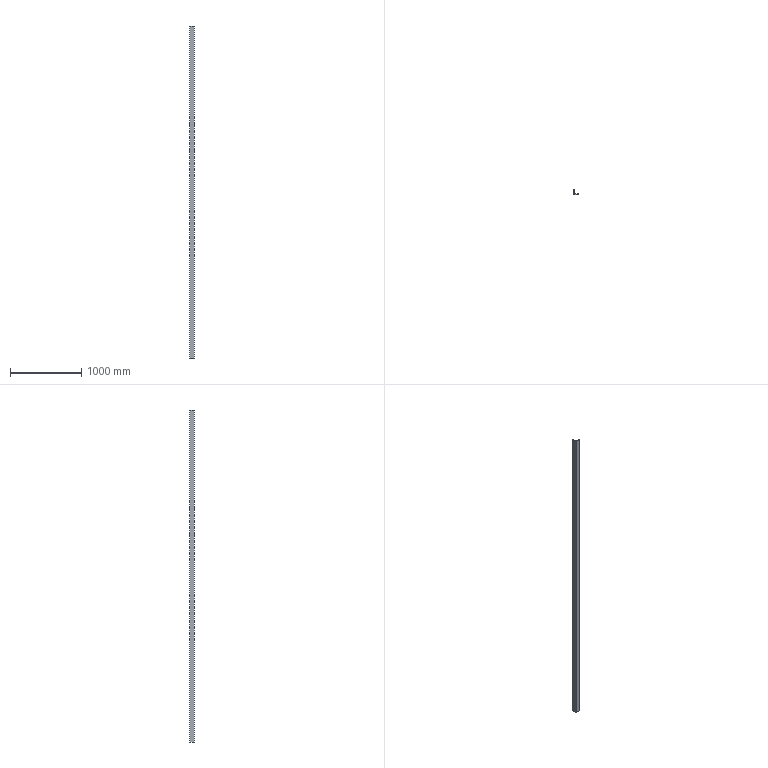Part | SolidWorks | features Extrusion 1 | 1 solid | 11 faces | box 70 x 70 x 4660 mm | volume 4966962 mm3 | plane 8 | cylinder 3 | commonest cylinder face diameters 6 x2 16 x1
STEP:
#1=CARTESIAN_POINT('',(5.,70.,0.));
#2=VERTEX_POINT('',#1);
#3=CARTESIAN_POINT('',(0.,70.,0.));
#4=VERTEX_POINT('',#3);
#5=CARTESIAN_POINT('',(5.,70.,0.));
#6=DIRECTION('',(-1.,0.,0.));
#7=VECTOR('',#6,1000.);
#8=LINE('',#5,#7);
#9=EDGE_CURVE('',#2,#4,#8,.T.);
#10=ORIENTED_EDGE('',*,*,#9,.T.);
#11=CARTESIAN_POINT('',(0.,70.,4660.));
#12=VERTEX_POINT('',#11);
#13=CARTESIAN_POINT('',(0.,70.,4660.));
#14=DIRECTION('',(0.,0.,-1.));
#15=VECTOR('',#14,1000.);
#16=LINE('',#13,#15);
#17=EDGE_CURVE('',#12,#4,#16,.T.);
#18=ORIENTED_EDGE('',*,*,#17,.F.);
#19=CARTESIAN_POINT('',(5.,70.,4660.));
#20=VERTEX_POINT('',#19);
#21=CARTESIAN_POINT('',(5.,70.,4660.));
#22=DIRECTION('',(-1.,0.,0.));
#23=VECTOR('',#22,1000.);
#24=LINE('',#21,#23);
#25=EDGE_CURVE('',#20,#12,#24,.T.);
#26=ORIENTED_EDGE('',*,*,#25,.F.);
#27=CARTESIAN_POINT('',(5.,70.,4660.));
#28=DIRECTION('',(0.,0.,-1.));
#29=VECTOR('',#28,1000.);
#30=LINE('',#27,#29);
#31=EDGE_CURVE('',#20,#2,#30,.T.);
#32=ORIENTED_EDGE('',*,*,#31,.T.);
#33=EDGE_LOOP('',(#10,#18,#26,#32));
#34=FACE_OUTER_BOUND('',#33,.T.);
#35=CARTESIAN_POINT('',(5.,70.,4660.));
#36=DIRECTION('',(0.,-1.,0.));
#37=DIRECTION('',(0.,0.,-1.));
#38=AXIS2_PLACEMENT_3D('',#35,#36,#37);
#39=PLANE('',#38);
#40=ADVANCED_FACE('',(#34),#39,.F.);
#41=CARTESIAN_POINT('',(0.,0.,0.));
#42=VERTEX_POINT('',#41);
#43=CARTESIAN_POINT('',(0.,70.,0.));
#44=DIRECTION('',(0.,-1.,0.));
#45=VECTOR('',#44,1000.);
#46=LINE('',#43,#45);
#47=EDGE_CURVE('',#4,#42,#46,.T.);
#48=ORIENTED_EDGE('',*,*,#47,.T.);
#49=CARTESIAN_POINT('',(0.,0.,4660.));
#50=VERTEX_POINT('',#49);
#51=CARTESIAN_POINT('',(0.,0.,4660.));
#52=DIRECTION('',(0.,0.,-1.));
#53=VECTOR('',#52,1000.);
#54=LINE('',#51,#53);
#55=EDGE_CURVE('',#50,#42,#54,.T.);
#56=ORIENTED_EDGE('',*,*,#55,.F.);
#57=CARTESIAN_POINT('',(0.,70.,4660.));
#58=DIRECTION('',(0.,-1.,0.));
#59=VECTOR('',#58,1000.);
#60=LINE('',#57,#59);
#61=EDGE_CURVE('',#12,#50,#60,.T.);
#62=ORIENTED_EDGE('',*,*,#61,.F.);
#63=ORIENTED_EDGE('',*,*,#17,.T.);
#64=EDGE_LOOP('',(#48,#56,#62,#63));
#65=FACE_OUTER_BOUND('',#64,.T.);
#66=CARTESIAN_POINT('',(0.,70.,4660.));
#67=DIRECTION('',(1.,0.,0.));
#68=DIRECTION('',(0.,0.,-1.));
#69=AXIS2_PLACEMENT_3D('',#66,#67,#68);
#70=PLANE('',#69);
#71=ADVANCED_FACE('',(#65),#70,.F.);
#72=CARTESIAN_POINT('',(70.,0.,0.));
#73=VERTEX_POINT('',#72);
#74=CARTESIAN_POINT('',(0.,0.,0.));
#75=DIRECTION('',(1.,0.,0.));
#76=VECTOR('',#75,1000.);
#77=LINE('',#74,#76);
#78=EDGE_CURVE('',#42,#73,#77,.T.);
#79=ORIENTED_EDGE('',*,*,#78,.T.);
#80=CARTESIAN_POINT('',(70.,0.,4660.));
#81=VERTEX_POINT('',#80);
#82=CARTESIAN_POINT('',(70.,0.,4660.));
#83=DIRECTION('',(0.,0.,-1.));
#84=VECTOR('',#83,1000.);
#85=LINE('',#82,#84);
#86=EDGE_CURVE('',#81,#73,#85,.T.);
#87=ORIENTED_EDGE('',*,*,#86,.F.);
#88=CARTESIAN_POINT('',(0.,0.,4660.));
#89=DIRECTION('',(1.,0.,0.));
#90=VECTOR('',#89,1000.);
#91=LINE('',#88,#90);
#92=EDGE_CURVE('',#50,#81,#91,.T.);
#93=ORIENTED_EDGE('',*,*,#92,.F.);
#94=ORIENTED_EDGE('',*,*,#55,.T.);
#95=EDGE_LOOP('',(#79,#87,#93,#94));
#96=FACE_OUTER_BOUND('',#95,.T.);
#97=CARTESIAN_POINT('',(0.,0.,4660.));
#98=DIRECTION('',(0.,1.,0.));
#99=DIRECTION('',(0.,0.,1.));
#100=AXIS2_PLACEMENT_3D('',#97,#98,#99);
#101=PLANE('',#100);
#102=ADVANCED_FACE('',(#96),#101,.F.);
#103=CARTESIAN_POINT('',(70.,5.,0.));
#104=VERTEX_POINT('',#103);
#105=CARTESIAN_POINT('',(70.,0.,0.));
#106=DIRECTION('',(0.,1.,0.));
#107=VECTOR('',#106,1000.);
#108=LINE('',#105,#107);
#109=EDGE_CURVE('',#73,#104,#108,.T.);
#110=ORIENTED_EDGE('',*,*,#109,.T.);
#111=CARTESIAN_POINT('',(70.,5.,4660.));
#112=VERTEX_POINT('',#111);
#113=CARTESIAN_POINT('',(70.,5.,4660.));
#114=DIRECTION('',(0.,0.,-1.));
#115=VECTOR('',#114,1000.);
#116=LINE('',#113,#115);
#117=EDGE_CURVE('',#112,#104,#116,.T.);
#118=ORIENTED_EDGE('',*,*,#117,.F.);
#119=CARTESIAN_POINT('',(70.,0.,4660.));
#120=DIRECTION('',(0.,1.,0.));
#121=VECTOR('',#120,1000.);
#122=LINE('',#119,#121);
#123=EDGE_CURVE('',#81,#112,#122,.T.);
#124=ORIENTED_EDGE('',*,*,#123,.F.);
#125=ORIENTED_EDGE('',*,*,#86,.T.);
#126=EDGE_LOOP('',(#110,#118,#124,#125));
#127=FACE_OUTER_BOUND('',#126,.T.);
#128=CARTESIAN_POINT('',(70.,0.,4660.));
#129=DIRECTION('',(-1.,0.,0.));
#130=DIRECTION('',(0.,0.,1.));
#131=AXIS2_PLACEMENT_3D('',#128,#129,#130);
#132=PLANE('',#131);
#133=ADVANCED_FACE('',(#127),#132,.F.);
#134=CARTESIAN_POINT('',(67.,8.,0.));
#135=VERTEX_POINT('',#134);
#136=CARTESIAN_POINT('',(67.,5.,0.));
#137=DIRECTION('',(0.,0.,1.));
#138=DIRECTION('',(1.,0.,0.));
#139=AXIS2_PLACEMENT_3D('',#136,#137,#138);
#140=CIRCLE('',#139,3.);
#141=EDGE_CURVE('',#104,#135,#140,.T.);
#142=ORIENTED_EDGE('',*,*,#141,.T.);
#143=CARTESIAN_POINT('',(67.,8.,4660.));
#144=VERTEX_POINT('',#143);
#145=CARTESIAN_POINT('',(67.,8.,4660.));
#146=DIRECTION('',(0.,0.,-1.));
#147=VECTOR('',#146,1000.);
#148=LINE('',#145,#147);
#149=EDGE_CURVE('',#144,#135,#148,.T.);
#150=ORIENTED_EDGE('',*,*,#149,.F.);
#151=CARTESIAN_POINT('',(67.,5.,4660.));
#152=DIRECTION('',(0.,0.,1.));
#153=DIRECTION('',(1.,0.,0.));
#154=AXIS2_PLACEMENT_3D('',#151,#152,#153);
#155=CIRCLE('',#154,3.);
#156=EDGE_CURVE('',#112,#144,#155,.T.);
#157=ORIENTED_EDGE('',*,*,#156,.F.);
#158=ORIENTED_EDGE('',*,*,#117,.T.);
#159=EDGE_LOOP('',(#142,#150,#157,#158));
#160=FACE_OUTER_BOUND('',#159,.T.);
#161=CARTESIAN_POINT('',(67.,5.,4660.));
#162=DIRECTION('',(0.,0.,-1.));
#163=DIRECTION('',(-1.,0.,0.));
#164=AXIS2_PLACEMENT_3D('',#161,#162,#163);
#165=CYLINDRICAL_SURFACE('',#164,3.);
#166=ADVANCED_FACE('',(#160),#165,.T.);
#167=CARTESIAN_POINT('',(16.,8.,0.));
#168=VERTEX_POINT('',#167);
#169=CARTESIAN_POINT('',(67.,8.,0.));
#170=DIRECTION('',(-1.,0.,0.));
#171=VECTOR('',#170,1000.);
#172=LINE('',#169,#171);
#173=EDGE_CURVE('',#135,#168,#172,.T.);
#174=ORIENTED_EDGE('',*,*,#173,.T.);
#175=CARTESIAN_POINT('',(16.,8.,4660.));
#176=VERTEX_POINT('',#175);
#177=CARTESIAN_POINT('',(16.,8.,4660.));
#178=DIRECTION('',(0.,0.,-1.));
#179=VECTOR('',#178,1000.);
#180=LINE('',#177,#179);
#181=EDGE_CURVE('',#176,#168,#180,.T.);
#182=ORIENTED_EDGE('',*,*,#181,.F.);
#183=CARTESIAN_POINT('',(67.,8.,4660.));
#184=DIRECTION('',(-1.,0.,0.));
#185=VECTOR('',#184,1000.);
#186=LINE('',#183,#185);
#187=EDGE_CURVE('',#144,#176,#186,.T.);
#188=ORIENTED_EDGE('',*,*,#187,.F.);
#189=ORIENTED_EDGE('',*,*,#149,.T.);
#190=EDGE_LOOP('',(#174,#182,#188,#189));
#191=FACE_OUTER_BOUND('',#190,.T.);
#192=CARTESIAN_POINT('',(67.,8.,4660.));
#193=DIRECTION('',(0.,-1.,0.));
#194=DIRECTION('',(1.,0.,0.));
#195=AXIS2_PLACEMENT_3D('',#192,#193,#194);
#196=PLANE('',#195);
#197=ADVANCED_FACE('',(#191),#196,.F.);
#198=CARTESIAN_POINT('',(8.,16.,0.));
#199=VERTEX_POINT('',#198);
#200=CARTESIAN_POINT('',(16.,16.,0.));
#201=DIRECTION('',(0.,0.,-1.));
#202=DIRECTION('',(-1.,0.,0.));
#203=AXIS2_PLACEMENT_3D('',#200,#201,#202);
#204=CIRCLE('',#203,8.);
#205=EDGE_CURVE('',#168,#199,#204,.T.);
#206=ORIENTED_EDGE('',*,*,#205,.T.);
#207=CARTESIAN_POINT('',(8.,16.,4660.));
#208=VERTEX_POINT('',#207);
#209=CARTESIAN_POINT('',(8.,16.,4660.));
#210=DIRECTION('',(0.,0.,-1.));
#211=VECTOR('',#210,1000.);
#212=LINE('',#209,#211);
#213=EDGE_CURVE('',#208,#199,#212,.T.);
#214=ORIENTED_EDGE('',*,*,#213,.F.);
#215=CARTESIAN_POINT('',(16.,16.,4660.));
#216=DIRECTION('',(0.,0.,-1.));
#217=DIRECTION('',(-1.,0.,0.));
#218=AXIS2_PLACEMENT_3D('',#215,#216,#217);
#219=CIRCLE('',#218,8.);
#220=EDGE_CURVE('',#176,#208,#219,.T.);
#221=ORIENTED_EDGE('',*,*,#220,.F.);
#222=ORIENTED_EDGE('',*,*,#181,.T.);
#223=EDGE_LOOP('',(#206,#214,#221,#222));
#224=FACE_OUTER_BOUND('',#223,.T.);
#225=CARTESIAN_POINT('',(16.,16.,4660.));
#226=DIRECTION('',(0.,0.,-1.));
#227=DIRECTION('',(-1.,0.,0.));
#228=AXIS2_PLACEMENT_3D('',#225,#226,#227);
#229=CYLINDRICAL_SURFACE('',#228,8.);
#230=ADVANCED_FACE('',(#224),#229,.F.);
#231=CARTESIAN_POINT('',(8.,67.,0.));
#232=VERTEX_POINT('',#231);
#233=CARTESIAN_POINT('',(8.,16.,0.));
#234=DIRECTION('',(0.,1.,0.));
#235=VECTOR('',#234,1000.);
#236=LINE('',#233,#235);
#237=EDGE_CURVE('',#199,#232,#236,.T.);
#238=ORIENTED_EDGE('',*,*,#237,.T.);
#239=CARTESIAN_POINT('',(8.,67.,4660.));
#240=VERTEX_POINT('',#239);
#241=CARTESIAN_POINT('',(8.,67.,4660.));
#242=DIRECTION('',(0.,0.,-1.));
#243=VECTOR('',#242,1000.);
#244=LINE('',#241,#243);
#245=EDGE_CURVE('',#240,#232,#244,.T.);
#246=ORIENTED_EDGE('',*,*,#245,.F.);
#247=CARTESIAN_POINT('',(8.,16.,4660.));
#248=DIRECTION('',(0.,1.,0.));
#249=VECTOR('',#248,1000.);
#250=LINE('',#247,#249);
#251=EDGE_CURVE('',#208,#240,#250,.T.);
#252=ORIENTED_EDGE('',*,*,#251,.F.);
#253=ORIENTED_EDGE('',*,*,#213,.T.);
#254=EDGE_LOOP('',(#238,#246,#252,#253));
#255=FACE_OUTER_BOUND('',#254,.T.);
#256=CARTESIAN_POINT('',(8.,16.,4660.));
#257=DIRECTION('',(-1.,0.,0.));
#258=DIRECTION('',(0.,-1.,0.));
#259=AXIS2_PLACEMENT_3D('',#256,#257,#258);
#260=PLANE('',#259);
#261=ADVANCED_FACE('',(#255),#260,.F.);
#262=CARTESIAN_POINT('',(5.,67.,0.));
#263=DIRECTION('',(0.,0.,1.));
#264=DIRECTION('',(1.,0.,0.));
#265=AXIS2_PLACEMENT_3D('',#262,#263,#264);
#266=CIRCLE('',#265,3.);
#267=EDGE_CURVE('',#232,#2,#266,.T.);
#268=ORIENTED_EDGE('',*,*,#267,.T.);
#269=ORIENTED_EDGE('',*,*,#31,.F.);
#270=CARTESIAN_POINT('',(5.,67.,4660.));
#271=DIRECTION('',(0.,0.,1.));
#272=DIRECTION('',(1.,0.,0.));
#273=AXIS2_PLACEMENT_3D('',#270,#271,#272);
#274=CIRCLE('',#273,3.);
#275=EDGE_CURVE('',#240,#20,#274,.T.);
#276=ORIENTED_EDGE('',*,*,#275,.F.);
#277=ORIENTED_EDGE('',*,*,#245,.T.);
#278=EDGE_LOOP('',(#268,#269,#276,#277));
#279=FACE_OUTER_BOUND('',#278,.T.);
#280=CARTESIAN_POINT('',(5.,67.,4660.));
#281=DIRECTION('',(0.,0.,-1.));
#282=DIRECTION('',(-1.,0.,0.));
#283=AXIS2_PLACEMENT_3D('',#280,#281,#282);
#284=CYLINDRICAL_SURFACE('',#283,3.);
#285=ADVANCED_FACE('',(#279),#284,.T.);
#286=ORIENTED_EDGE('',*,*,#25,.T.);
#287=ORIENTED_EDGE('',*,*,#61,.T.);
#288=ORIENTED_EDGE('',*,*,#92,.T.);
#289=ORIENTED_EDGE('',*,*,#123,.T.);
#290=ORIENTED_EDGE('',*,*,#156,.T.);
#291=ORIENTED_EDGE('',*,*,#187,.T.);
#292=ORIENTED_EDGE('',*,*,#220,.T.);
#293=ORIENTED_EDGE('',*,*,#251,.T.);
#294=ORIENTED_EDGE('',*,*,#275,.T.);
#295=EDGE_LOOP('',(#286,#287,#288,#289,#290,#291,#292,#293,#294));
#296=FACE_OUTER_BOUND('',#295,.T.);
#297=CARTESIAN_POINT('',(67.,5.,4660.));
#298=DIRECTION('',(0.,0.,1.));
#299=DIRECTION('',(1.,0.,0.));
#300=AXIS2_PLACEMENT_3D('',#297,#298,#299);
#301=PLANE('',#300);
#302=ADVANCED_FACE('',(#296),#301,.T.);
#303=ORIENTED_EDGE('',*,*,#9,.F.);
#304=ORIENTED_EDGE('',*,*,#267,.F.);
#305=ORIENTED_EDGE('',*,*,#237,.F.);
#306=ORIENTED_EDGE('',*,*,#205,.F.);
#307=ORIENTED_EDGE('',*,*,#173,.F.);
#308=ORIENTED_EDGE('',*,*,#141,.F.);
#309=ORIENTED_EDGE('',*,*,#109,.F.);
#310=ORIENTED_EDGE('',*,*,#78,.F.);
#311=ORIENTED_EDGE('',*,*,#47,.F.);
#312=EDGE_LOOP('',(#303,#304,#305,#306,#307,#308,#309,#310,#311));
#313=FACE_OUTER_BOUND('',#312,.T.);
#314=CARTESIAN_POINT('',(67.,5.,0.));
#315=DIRECTION('',(0.,0.,1.));
#316=DIRECTION('',(1.,0.,0.));
#317=AXIS2_PLACEMENT_3D('',#314,#315,#316);
#318=PLANE('',#317);
#319=ADVANCED_FACE('',(#313),#318,.F.);
#320=CLOSED_SHELL('',(#40,#71,#102,#133,#166,#197,#230,#261,#285,#302,#319));
#321=MANIFOLD_SOLID_BREP('',#320);
#322=CARTESIAN_POINT('',(0.,0.,0.));
#323=DIRECTION('',(0.,0.,1.));
#324=DIRECTION('',(1.,0.,0.));
#325=AXIS2_PLACEMENT_3D('',#322,#323,#324);
#326=(LENGTH_UNIT()NAMED_UNIT(*)SI_UNIT(.MILLI.,.METRE.));
#327=UNCERTAINTY_MEASURE_WITH_UNIT(LENGTH_MEASURE(0.00001),#326,'','');
#328=(NAMED_UNIT(*)PLANE_ANGLE_UNIT()SI_UNIT($,.RADIAN.));
#329=(NAMED_UNIT(*)SI_UNIT($,.STERADIAN.)SOLID_ANGLE_UNIT());
#330=(GEOMETRIC_REPRESENTATION_CONTEXT(3)GLOBAL_UNCERTAINTY_ASSIGNED_CONTEXT((#327))GLOBAL_UNIT_ASSIGNED_CONTEXT((#326,#328,#329))REPRESENTATION_CONTEXT('',''));
#331=ADVANCED_BREP_SHAPE_REPRESENTATION('',(#321,#325),#330);